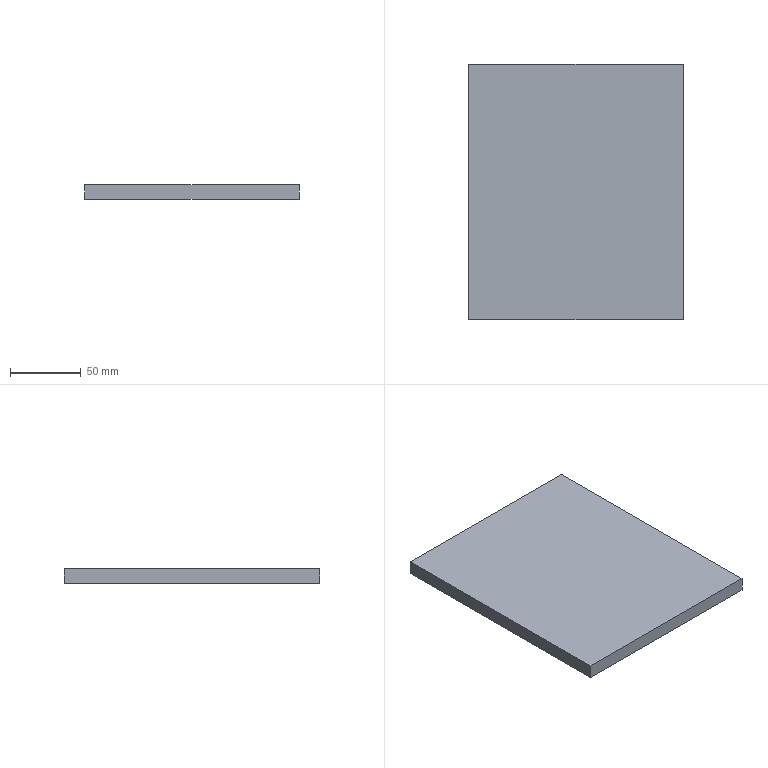Part | STEP file | 001-004-Feeding mechanism slide connecting plate | 1 solid | 6 faces | box 151 x 180 x 10 mm | volume 271800 mm3 | plane 6
STEP:
#1=CARTESIAN_POINT('',(0.,0.,0.));
#2=DIRECTION('',(0.,0.,1.));
#3=DIRECTION('',(1.,0.,0.));
#4=AXIS2_PLACEMENT_3D('',#1,#2,#3);
#5=CARTESIAN_POINT('',(75.5,-90.,0.));
#6=VERTEX_POINT('',#5);
#7=CARTESIAN_POINT('',(75.5,90.,0.));
#8=VERTEX_POINT('',#7);
#9=CARTESIAN_POINT('',(75.5,-90.,0.));
#10=DIRECTION('',(0.,1.,0.));
#11=VECTOR('',#10,1.);
#12=LINE('',#9,#11);
#13=CARTESIAN_POINT('',(75.5,-90.,10.));
#14=DIRECTION('',(-1.,0.,0.));
#15=DIRECTION('',(0.,0.,1.));
#16=AXIS2_PLACEMENT_3D('',#13,#14,#15);
#17=PLANE('',#16);
#18=CARTESIAN_POINT('',(-10.,0.));
#19=DIRECTION('',(0.,1.));
#20=VECTOR('',#19,1.);
#21=LINE('',#18,#20);
#22=(GEOMETRIC_REPRESENTATION_CONTEXT(2)PARAMETRIC_REPRESENTATION_CONTEXT()REPRESENTATION_CONTEXT('',''));
#23=DEFINITIONAL_REPRESENTATION('',(#21),#22);
#24=PCURVE('',#17,#23);
#25=CARTESIAN_POINT('',(0.,0.,0.));
#26=DIRECTION('',(0.,0.,-1.));
#27=DIRECTION('',(-1.,0.,0.));
#28=AXIS2_PLACEMENT_3D('',#25,#26,#27);
#29=PLANE('',#28);
#30=CARTESIAN_POINT('',(-75.5,-90.));
#31=DIRECTION('',(0.,1.));
#32=VECTOR('',#31,1.);
#33=LINE('',#30,#32);
#34=(GEOMETRIC_REPRESENTATION_CONTEXT(2)PARAMETRIC_REPRESENTATION_CONTEXT()REPRESENTATION_CONTEXT('',''));
#35=DEFINITIONAL_REPRESENTATION('',(#33),#34);
#36=PCURVE('',#29,#35);
#37=SURFACE_CURVE('',#12,(#24,#36),.PCURVE_S1.);
#38=EDGE_CURVE('',#6,#8,#37,.T.);
#39=ORIENTED_EDGE('',*,*,#38,.T.);
#40=CARTESIAN_POINT('',(75.5,90.,10.));
#41=VERTEX_POINT('',#40);
#42=CARTESIAN_POINT('',(75.5,90.,10.));
#43=DIRECTION('',(0.,0.,-1.));
#44=VECTOR('',#43,1.);
#45=LINE('',#42,#44);
#46=CARTESIAN_POINT('',(0.,180.));
#47=DIRECTION('',(-1.,0.));
#48=VECTOR('',#47,1.);
#49=LINE('',#46,#48);
#50=(GEOMETRIC_REPRESENTATION_CONTEXT(2)PARAMETRIC_REPRESENTATION_CONTEXT()REPRESENTATION_CONTEXT('',''));
#51=DEFINITIONAL_REPRESENTATION('',(#49),#50);
#52=PCURVE('',#17,#51);
#53=CARTESIAN_POINT('',(-75.5,90.,10.));
#54=DIRECTION('',(0.,-1.,0.));
#55=DIRECTION('',(0.,0.,-1.));
#56=AXIS2_PLACEMENT_3D('',#53,#54,#55);
#57=PLANE('',#56);
#58=CARTESIAN_POINT('',(0.,151.));
#59=DIRECTION('',(1.,0.));
#60=VECTOR('',#59,1.);
#61=LINE('',#58,#60);
#62=(GEOMETRIC_REPRESENTATION_CONTEXT(2)PARAMETRIC_REPRESENTATION_CONTEXT()REPRESENTATION_CONTEXT('',''));
#63=DEFINITIONAL_REPRESENTATION('',(#61),#62);
#64=PCURVE('',#57,#63);
#65=SURFACE_CURVE('',#45,(#52,#64),.PCURVE_S1.);
#66=EDGE_CURVE('',#41,#8,#65,.T.);
#67=ORIENTED_EDGE('',*,*,#66,.F.);
#68=CARTESIAN_POINT('',(75.5,-90.,10.));
#69=VERTEX_POINT('',#68);
#70=CARTESIAN_POINT('',(75.5,-90.,10.));
#71=DIRECTION('',(0.,1.,0.));
#72=VECTOR('',#71,1.);
#73=LINE('',#70,#72);
#74=CARTESIAN_POINT('',(0.,0.));
#75=DIRECTION('',(0.,1.));
#76=VECTOR('',#75,1.);
#77=LINE('',#74,#76);
#78=(GEOMETRIC_REPRESENTATION_CONTEXT(2)PARAMETRIC_REPRESENTATION_CONTEXT()REPRESENTATION_CONTEXT('',''));
#79=DEFINITIONAL_REPRESENTATION('',(#77),#78);
#80=PCURVE('',#17,#79);
#81=CARTESIAN_POINT('',(0.,0.,10.));
#82=DIRECTION('',(0.,0.,-1.));
#83=DIRECTION('',(-1.,0.,0.));
#84=AXIS2_PLACEMENT_3D('',#81,#82,#83);
#85=PLANE('',#84);
#86=CARTESIAN_POINT('',(-75.5,-90.));
#87=DIRECTION('',(0.,1.));
#88=VECTOR('',#87,1.);
#89=LINE('',#86,#88);
#90=(GEOMETRIC_REPRESENTATION_CONTEXT(2)PARAMETRIC_REPRESENTATION_CONTEXT()REPRESENTATION_CONTEXT('',''));
#91=DEFINITIONAL_REPRESENTATION('',(#89),#90);
#92=PCURVE('',#85,#91);
#93=SURFACE_CURVE('',#73,(#80,#92),.PCURVE_S1.);
#94=EDGE_CURVE('',#69,#41,#93,.T.);
#95=ORIENTED_EDGE('',*,*,#94,.F.);
#96=CARTESIAN_POINT('',(75.5,-90.,10.));
#97=DIRECTION('',(0.,0.,-1.));
#98=VECTOR('',#97,1.);
#99=LINE('',#96,#98);
#100=CARTESIAN_POINT('',(0.,0.));
#101=DIRECTION('',(-1.,0.));
#102=VECTOR('',#101,1.);
#103=LINE('',#100,#102);
#104=(GEOMETRIC_REPRESENTATION_CONTEXT(2)PARAMETRIC_REPRESENTATION_CONTEXT()REPRESENTATION_CONTEXT('',''));
#105=DEFINITIONAL_REPRESENTATION('',(#103),#104);
#106=PCURVE('',#17,#105);
#107=CARTESIAN_POINT('',(-75.5,-90.,10.));
#108=DIRECTION('',(0.,1.,0.));
#109=DIRECTION('',(0.,0.,1.));
#110=AXIS2_PLACEMENT_3D('',#107,#108,#109);
#111=PLANE('',#110);
#112=CARTESIAN_POINT('',(0.,151.));
#113=DIRECTION('',(-1.,0.));
#114=VECTOR('',#113,1.);
#115=LINE('',#112,#114);
#116=(GEOMETRIC_REPRESENTATION_CONTEXT(2)PARAMETRIC_REPRESENTATION_CONTEXT()REPRESENTATION_CONTEXT('',''));
#117=DEFINITIONAL_REPRESENTATION('',(#115),#116);
#118=PCURVE('',#111,#117);
#119=SURFACE_CURVE('',#99,(#106,#118),.PCURVE_S1.);
#120=EDGE_CURVE('',#69,#6,#119,.T.);
#121=ORIENTED_EDGE('',*,*,#120,.T.);
#122=EDGE_LOOP('',(#39,#67,#95,#121));
#123=FACE_BOUND('',#122,.T.);
#124=ADVANCED_FACE('',(#123),#17,.F.);
#125=CARTESIAN_POINT('',(-75.5,90.,0.));
#126=VERTEX_POINT('',#125);
#127=CARTESIAN_POINT('',(-75.5,90.,0.));
#128=DIRECTION('',(-1.,0.,0.));
#129=VECTOR('',#128,1.);
#130=LINE('',#127,#129);
#131=CARTESIAN_POINT('',(10.,0.));
#132=DIRECTION('',(0.,-1.));
#133=VECTOR('',#132,1.);
#134=LINE('',#131,#133);
#135=(GEOMETRIC_REPRESENTATION_CONTEXT(2)PARAMETRIC_REPRESENTATION_CONTEXT()REPRESENTATION_CONTEXT('',''));
#136=DEFINITIONAL_REPRESENTATION('',(#134),#135);
#137=PCURVE('',#57,#136);
#138=CARTESIAN_POINT('',(75.5,90.));
#139=DIRECTION('',(1.,0.));
#140=VECTOR('',#139,1.);
#141=LINE('',#138,#140);
#142=(GEOMETRIC_REPRESENTATION_CONTEXT(2)PARAMETRIC_REPRESENTATION_CONTEXT()REPRESENTATION_CONTEXT('',''));
#143=DEFINITIONAL_REPRESENTATION('',(#141),#142);
#144=PCURVE('',#29,#143);
#145=SURFACE_CURVE('',#130,(#137,#144),.PCURVE_S1.);
#146=EDGE_CURVE('',#8,#126,#145,.T.);
#147=ORIENTED_EDGE('',*,*,#146,.T.);
#148=CARTESIAN_POINT('',(-75.5,90.,10.));
#149=VERTEX_POINT('',#148);
#150=CARTESIAN_POINT('',(-75.5,90.,10.));
#151=DIRECTION('',(0.,0.,-1.));
#152=VECTOR('',#151,1.);
#153=LINE('',#150,#152);
#154=CARTESIAN_POINT('',(0.,0.));
#155=DIRECTION('',(1.,0.));
#156=VECTOR('',#155,1.);
#157=LINE('',#154,#156);
#158=(GEOMETRIC_REPRESENTATION_CONTEXT(2)PARAMETRIC_REPRESENTATION_CONTEXT()REPRESENTATION_CONTEXT('',''));
#159=DEFINITIONAL_REPRESENTATION('',(#157),#158);
#160=PCURVE('',#57,#159);
#161=CARTESIAN_POINT('',(-75.5,-90.,10.));
#162=DIRECTION('',(1.,0.,0.));
#163=DIRECTION('',(0.,0.,-1.));
#164=AXIS2_PLACEMENT_3D('',#161,#162,#163);
#165=PLANE('',#164);
#166=CARTESIAN_POINT('',(0.,180.));
#167=DIRECTION('',(1.,0.));
#168=VECTOR('',#167,1.);
#169=LINE('',#166,#168);
#170=(GEOMETRIC_REPRESENTATION_CONTEXT(2)PARAMETRIC_REPRESENTATION_CONTEXT()REPRESENTATION_CONTEXT('',''));
#171=DEFINITIONAL_REPRESENTATION('',(#169),#170);
#172=PCURVE('',#165,#171);
#173=SURFACE_CURVE('',#153,(#160,#172),.PCURVE_S1.);
#174=EDGE_CURVE('',#149,#126,#173,.T.);
#175=ORIENTED_EDGE('',*,*,#174,.F.);
#176=CARTESIAN_POINT('',(-75.5,90.,10.));
#177=DIRECTION('',(-1.,0.,0.));
#178=VECTOR('',#177,1.);
#179=LINE('',#176,#178);
#180=CARTESIAN_POINT('',(0.,0.));
#181=DIRECTION('',(0.,-1.));
#182=VECTOR('',#181,1.);
#183=LINE('',#180,#182);
#184=(GEOMETRIC_REPRESENTATION_CONTEXT(2)PARAMETRIC_REPRESENTATION_CONTEXT()REPRESENTATION_CONTEXT('',''));
#185=DEFINITIONAL_REPRESENTATION('',(#183),#184);
#186=PCURVE('',#57,#185);
#187=CARTESIAN_POINT('',(75.5,90.));
#188=DIRECTION('',(1.,0.));
#189=VECTOR('',#188,1.);
#190=LINE('',#187,#189);
#191=(GEOMETRIC_REPRESENTATION_CONTEXT(2)PARAMETRIC_REPRESENTATION_CONTEXT()REPRESENTATION_CONTEXT('',''));
#192=DEFINITIONAL_REPRESENTATION('',(#190),#191);
#193=PCURVE('',#85,#192);
#194=SURFACE_CURVE('',#179,(#186,#193),.PCURVE_S1.);
#195=EDGE_CURVE('',#41,#149,#194,.T.);
#196=ORIENTED_EDGE('',*,*,#195,.F.);
#197=ORIENTED_EDGE('',*,*,#66,.T.);
#198=EDGE_LOOP('',(#147,#175,#196,#197));
#199=FACE_BOUND('',#198,.T.);
#200=ADVANCED_FACE('',(#199),#57,.F.);
#201=CARTESIAN_POINT('',(-75.5,-90.,0.));
#202=VERTEX_POINT('',#201);
#203=CARTESIAN_POINT('',(-75.5,-90.,0.));
#204=DIRECTION('',(0.,-1.,0.));
#205=VECTOR('',#204,1.);
#206=LINE('',#203,#205);
#207=CARTESIAN_POINT('',(10.,0.));
#208=DIRECTION('',(0.,-1.));
#209=VECTOR('',#208,1.);
#210=LINE('',#207,#209);
#211=(GEOMETRIC_REPRESENTATION_CONTEXT(2)PARAMETRIC_REPRESENTATION_CONTEXT()REPRESENTATION_CONTEXT('',''));
#212=DEFINITIONAL_REPRESENTATION('',(#210),#211);
#213=PCURVE('',#165,#212);
#214=CARTESIAN_POINT('',(75.5,-90.));
#215=DIRECTION('',(0.,-1.));
#216=VECTOR('',#215,1.);
#217=LINE('',#214,#216);
#218=(GEOMETRIC_REPRESENTATION_CONTEXT(2)PARAMETRIC_REPRESENTATION_CONTEXT()REPRESENTATION_CONTEXT('',''));
#219=DEFINITIONAL_REPRESENTATION('',(#217),#218);
#220=PCURVE('',#29,#219);
#221=SURFACE_CURVE('',#206,(#213,#220),.PCURVE_S1.);
#222=EDGE_CURVE('',#126,#202,#221,.T.);
#223=ORIENTED_EDGE('',*,*,#222,.T.);
#224=CARTESIAN_POINT('',(-75.5,-90.,10.));
#225=VERTEX_POINT('',#224);
#226=CARTESIAN_POINT('',(-75.5,-90.,10.));
#227=DIRECTION('',(0.,0.,-1.));
#228=VECTOR('',#227,1.);
#229=LINE('',#226,#228);
#230=CARTESIAN_POINT('',(0.,0.));
#231=DIRECTION('',(1.,0.));
#232=VECTOR('',#231,1.);
#233=LINE('',#230,#232);
#234=(GEOMETRIC_REPRESENTATION_CONTEXT(2)PARAMETRIC_REPRESENTATION_CONTEXT()REPRESENTATION_CONTEXT('',''));
#235=DEFINITIONAL_REPRESENTATION('',(#233),#234);
#236=PCURVE('',#165,#235);
#237=CARTESIAN_POINT('',(0.,0.));
#238=DIRECTION('',(-1.,0.));
#239=VECTOR('',#238,1.);
#240=LINE('',#237,#239);
#241=(GEOMETRIC_REPRESENTATION_CONTEXT(2)PARAMETRIC_REPRESENTATION_CONTEXT()REPRESENTATION_CONTEXT('',''));
#242=DEFINITIONAL_REPRESENTATION('',(#240),#241);
#243=PCURVE('',#111,#242);
#244=SURFACE_CURVE('',#229,(#236,#243),.PCURVE_S1.);
#245=EDGE_CURVE('',#225,#202,#244,.T.);
#246=ORIENTED_EDGE('',*,*,#245,.F.);
#247=CARTESIAN_POINT('',(-75.5,-90.,10.));
#248=DIRECTION('',(0.,-1.,0.));
#249=VECTOR('',#248,1.);
#250=LINE('',#247,#249);
#251=CARTESIAN_POINT('',(0.,0.));
#252=DIRECTION('',(0.,-1.));
#253=VECTOR('',#252,1.);
#254=LINE('',#251,#253);
#255=(GEOMETRIC_REPRESENTATION_CONTEXT(2)PARAMETRIC_REPRESENTATION_CONTEXT()REPRESENTATION_CONTEXT('',''));
#256=DEFINITIONAL_REPRESENTATION('',(#254),#255);
#257=PCURVE('',#165,#256);
#258=CARTESIAN_POINT('',(75.5,-90.));
#259=DIRECTION('',(0.,-1.));
#260=VECTOR('',#259,1.);
#261=LINE('',#258,#260);
#262=(GEOMETRIC_REPRESENTATION_CONTEXT(2)PARAMETRIC_REPRESENTATION_CONTEXT()REPRESENTATION_CONTEXT('',''));
#263=DEFINITIONAL_REPRESENTATION('',(#261),#262);
#264=PCURVE('',#85,#263);
#265=SURFACE_CURVE('',#250,(#257,#264),.PCURVE_S1.);
#266=EDGE_CURVE('',#149,#225,#265,.T.);
#267=ORIENTED_EDGE('',*,*,#266,.F.);
#268=ORIENTED_EDGE('',*,*,#174,.T.);
#269=EDGE_LOOP('',(#223,#246,#267,#268));
#270=FACE_BOUND('',#269,.T.);
#271=ADVANCED_FACE('',(#270),#165,.F.);
#272=CARTESIAN_POINT('',(-75.5,-90.,0.));
#273=DIRECTION('',(1.,0.,0.));
#274=VECTOR('',#273,1.);
#275=LINE('',#272,#274);
#276=CARTESIAN_POINT('',(-10.,0.));
#277=DIRECTION('',(0.,1.));
#278=VECTOR('',#277,1.);
#279=LINE('',#276,#278);
#280=(GEOMETRIC_REPRESENTATION_CONTEXT(2)PARAMETRIC_REPRESENTATION_CONTEXT()REPRESENTATION_CONTEXT('',''));
#281=DEFINITIONAL_REPRESENTATION('',(#279),#280);
#282=PCURVE('',#111,#281);
#283=CARTESIAN_POINT('',(75.5,-90.));
#284=DIRECTION('',(-1.,0.));
#285=VECTOR('',#284,1.);
#286=LINE('',#283,#285);
#287=(GEOMETRIC_REPRESENTATION_CONTEXT(2)PARAMETRIC_REPRESENTATION_CONTEXT()REPRESENTATION_CONTEXT('',''));
#288=DEFINITIONAL_REPRESENTATION('',(#286),#287);
#289=PCURVE('',#29,#288);
#290=SURFACE_CURVE('',#275,(#282,#289),.PCURVE_S1.);
#291=EDGE_CURVE('',#202,#6,#290,.T.);
#292=ORIENTED_EDGE('',*,*,#291,.T.);
#293=ORIENTED_EDGE('',*,*,#120,.F.);
#294=CARTESIAN_POINT('',(-75.5,-90.,10.));
#295=DIRECTION('',(1.,0.,0.));
#296=VECTOR('',#295,1.);
#297=LINE('',#294,#296);
#298=CARTESIAN_POINT('',(0.,0.));
#299=DIRECTION('',(0.,1.));
#300=VECTOR('',#299,1.);
#301=LINE('',#298,#300);
#302=(GEOMETRIC_REPRESENTATION_CONTEXT(2)PARAMETRIC_REPRESENTATION_CONTEXT()REPRESENTATION_CONTEXT('',''));
#303=DEFINITIONAL_REPRESENTATION('',(#301),#302);
#304=PCURVE('',#111,#303);
#305=CARTESIAN_POINT('',(75.5,-90.));
#306=DIRECTION('',(-1.,0.));
#307=VECTOR('',#306,1.);
#308=LINE('',#305,#307);
#309=(GEOMETRIC_REPRESENTATION_CONTEXT(2)PARAMETRIC_REPRESENTATION_CONTEXT()REPRESENTATION_CONTEXT('',''));
#310=DEFINITIONAL_REPRESENTATION('',(#308),#309);
#311=PCURVE('',#85,#310);
#312=SURFACE_CURVE('',#297,(#304,#311),.PCURVE_S1.);
#313=EDGE_CURVE('',#225,#69,#312,.T.);
#314=ORIENTED_EDGE('',*,*,#313,.F.);
#315=ORIENTED_EDGE('',*,*,#245,.T.);
#316=EDGE_LOOP('',(#292,#293,#314,#315));
#317=FACE_BOUND('',#316,.T.);
#318=ADVANCED_FACE('',(#317),#111,.F.);
#319=ORIENTED_EDGE('',*,*,#94,.T.);
#320=ORIENTED_EDGE('',*,*,#195,.T.);
#321=ORIENTED_EDGE('',*,*,#266,.T.);
#322=ORIENTED_EDGE('',*,*,#313,.T.);
#323=EDGE_LOOP('',(#319,#320,#321,#322));
#324=FACE_BOUND('',#323,.T.);
#325=ADVANCED_FACE('',(#324),#85,.F.);
#326=ORIENTED_EDGE('',*,*,#38,.F.);
#327=ORIENTED_EDGE('',*,*,#291,.F.);
#328=ORIENTED_EDGE('',*,*,#222,.F.);
#329=ORIENTED_EDGE('',*,*,#146,.F.);
#330=EDGE_LOOP('',(#326,#327,#328,#329));
#331=FACE_BOUND('',#330,.T.);
#332=ADVANCED_FACE('',(#331),#29,.T.);
#333=CLOSED_SHELL('',(#124,#200,#271,#318,#325,#332));
#334=MANIFOLD_SOLID_BREP('',#333);
#335=(LENGTH_UNIT()NAMED_UNIT(*)SI_UNIT(.MILLI.,.METRE.));
#336=UNCERTAINTY_MEASURE_WITH_UNIT(LENGTH_MEASURE(0.0000001),#335,'','');
#337=(NAMED_UNIT(*)PLANE_ANGLE_UNIT()SI_UNIT($,.RADIAN.));
#338=(NAMED_UNIT(*)SI_UNIT($,.STERADIAN.)SOLID_ANGLE_UNIT());
#339=(GEOMETRIC_REPRESENTATION_CONTEXT(3)GLOBAL_UNCERTAINTY_ASSIGNED_CONTEXT((#336))GLOBAL_UNIT_ASSIGNED_CONTEXT((#335,#337,#338))REPRESENTATION_CONTEXT('',''));
#340=ADVANCED_BREP_SHAPE_REPRESENTATION('',(#4,#334),#339);